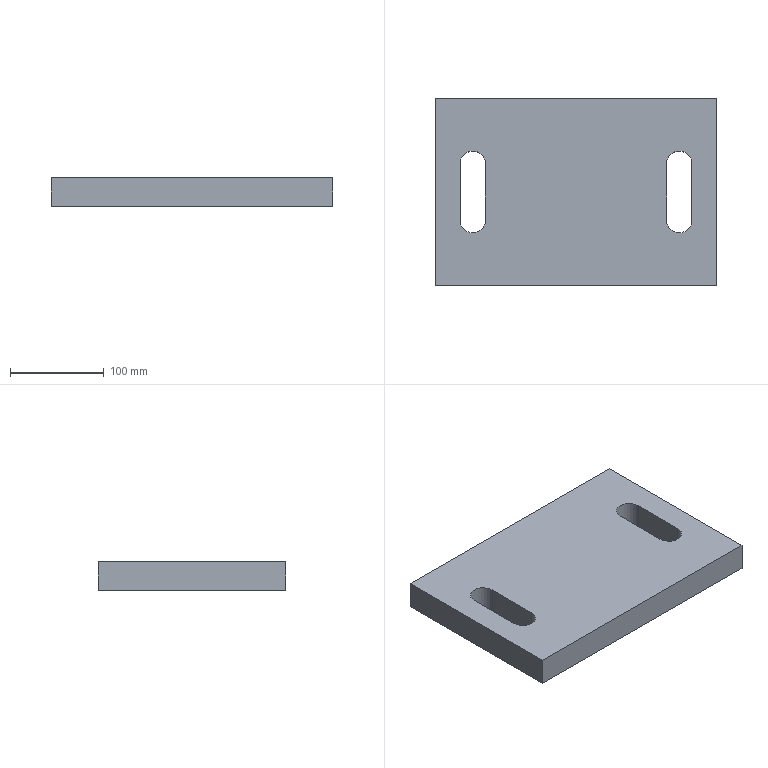Part | SolidWorks | features Extrusion 1 | 1 solid | 14 faces | box 300 x 200 x 30 mm | volume 1668447 mm3 | plane 10 | cylinder 4 | commonest cylinder face diameters 27 x4
STEP:
#1=CARTESIAN_POINT('',(273.5,130.,30.));
#2=VERTEX_POINT('',#1);
#3=CARTESIAN_POINT('',(246.5,130.,30.));
#4=VERTEX_POINT('',#3);
#5=CARTESIAN_POINT('',(260.,130.,30.));
#6=DIRECTION('',(0.,0.,1.));
#7=DIRECTION('',(1.,0.,0.));
#8=AXIS2_PLACEMENT_3D('',#5,#6,#7);
#9=CIRCLE('',#8,13.5);
#10=EDGE_CURVE('',#2,#4,#9,.T.);
#11=ORIENTED_EDGE('',*,*,#10,.F.);
#12=CARTESIAN_POINT('',(273.5,70.,30.));
#13=VERTEX_POINT('',#12);
#14=CARTESIAN_POINT('',(273.5,130.,30.));
#15=DIRECTION('',(0.,1.,0.));
#16=VECTOR('',#15,1000.);
#17=LINE('',#14,#16);
#18=EDGE_CURVE('',#13,#2,#17,.T.);
#19=ORIENTED_EDGE('',*,*,#18,.F.);
#20=CARTESIAN_POINT('',(246.5,70.,30.));
#21=VERTEX_POINT('',#20);
#22=CARTESIAN_POINT('',(260.,70.,30.));
#23=DIRECTION('',(0.,0.,1.));
#24=DIRECTION('',(1.,0.,0.));
#25=AXIS2_PLACEMENT_3D('',#22,#23,#24);
#26=CIRCLE('',#25,13.5);
#27=EDGE_CURVE('',#21,#13,#26,.T.);
#28=ORIENTED_EDGE('',*,*,#27,.F.);
#29=CARTESIAN_POINT('',(246.5,130.,30.));
#30=DIRECTION('',(0.,-1.,0.));
#31=VECTOR('',#30,1000.);
#32=LINE('',#29,#31);
#33=EDGE_CURVE('',#4,#21,#32,.T.);
#34=ORIENTED_EDGE('',*,*,#33,.F.);
#35=EDGE_LOOP('',(#11,#19,#28,#34));
#36=FACE_BOUND('',#35,.T.);
#37=CARTESIAN_POINT('',(0.,200.,30.));
#38=VERTEX_POINT('',#37);
#39=CARTESIAN_POINT('',(0.,0.,30.));
#40=VERTEX_POINT('',#39);
#41=CARTESIAN_POINT('',(0.,0.,30.));
#42=DIRECTION('',(0.,-1.,0.));
#43=VECTOR('',#42,1000.);
#44=LINE('',#41,#43);
#45=EDGE_CURVE('',#38,#40,#44,.T.);
#46=ORIENTED_EDGE('',*,*,#45,.T.);
#47=CARTESIAN_POINT('',(300.,0.,30.));
#48=VERTEX_POINT('',#47);
#49=CARTESIAN_POINT('',(0.,0.,30.));
#50=DIRECTION('',(1.,0.,0.));
#51=VECTOR('',#50,1000.);
#52=LINE('',#49,#51);
#53=EDGE_CURVE('',#40,#48,#52,.T.);
#54=ORIENTED_EDGE('',*,*,#53,.T.);
#55=CARTESIAN_POINT('',(300.,200.,30.));
#56=VERTEX_POINT('',#55);
#57=CARTESIAN_POINT('',(300.,0.,30.));
#58=DIRECTION('',(0.,1.,0.));
#59=VECTOR('',#58,1000.);
#60=LINE('',#57,#59);
#61=EDGE_CURVE('',#48,#56,#60,.T.);
#62=ORIENTED_EDGE('',*,*,#61,.T.);
#63=CARTESIAN_POINT('',(0.,200.,30.));
#64=DIRECTION('',(-1.,0.,0.));
#65=VECTOR('',#64,1000.);
#66=LINE('',#63,#65);
#67=EDGE_CURVE('',#56,#38,#66,.T.);
#68=ORIENTED_EDGE('',*,*,#67,.T.);
#69=EDGE_LOOP('',(#46,#54,#62,#68));
#70=FACE_OUTER_BOUND('',#69,.T.);
#71=CARTESIAN_POINT('',(53.5,130.,30.));
#72=VERTEX_POINT('',#71);
#73=CARTESIAN_POINT('',(26.5,130.,30.));
#74=VERTEX_POINT('',#73);
#75=CARTESIAN_POINT('',(40.,130.,30.));
#76=DIRECTION('',(0.,0.,1.));
#77=DIRECTION('',(1.,0.,0.));
#78=AXIS2_PLACEMENT_3D('',#75,#76,#77);
#79=CIRCLE('',#78,13.5);
#80=EDGE_CURVE('',#72,#74,#79,.T.);
#81=ORIENTED_EDGE('',*,*,#80,.F.);
#82=CARTESIAN_POINT('',(53.5,70.,30.));
#83=VERTEX_POINT('',#82);
#84=CARTESIAN_POINT('',(53.5,130.,30.));
#85=DIRECTION('',(0.,1.,0.));
#86=VECTOR('',#85,1000.);
#87=LINE('',#84,#86);
#88=EDGE_CURVE('',#83,#72,#87,.T.);
#89=ORIENTED_EDGE('',*,*,#88,.F.);
#90=CARTESIAN_POINT('',(26.5,70.,30.));
#91=VERTEX_POINT('',#90);
#92=CARTESIAN_POINT('',(40.,70.,30.));
#93=DIRECTION('',(0.,0.,1.));
#94=DIRECTION('',(1.,0.,0.));
#95=AXIS2_PLACEMENT_3D('',#92,#93,#94);
#96=CIRCLE('',#95,13.5);
#97=EDGE_CURVE('',#91,#83,#96,.T.);
#98=ORIENTED_EDGE('',*,*,#97,.F.);
#99=CARTESIAN_POINT('',(26.5,130.,30.));
#100=DIRECTION('',(0.,-1.,0.));
#101=VECTOR('',#100,1000.);
#102=LINE('',#99,#101);
#103=EDGE_CURVE('',#74,#91,#102,.T.);
#104=ORIENTED_EDGE('',*,*,#103,.F.);
#105=EDGE_LOOP('',(#81,#89,#98,#104));
#106=FACE_BOUND('',#105,.T.);
#107=CARTESIAN_POINT('',(0.,0.,30.));
#108=DIRECTION('',(0.,0.,-1.));
#109=DIRECTION('',(-1.,0.,0.));
#110=AXIS2_PLACEMENT_3D('',#107,#108,#109);
#111=PLANE('',#110);
#112=ADVANCED_FACE('',(#36,#70,#106),#111,.F.);
#113=CARTESIAN_POINT('',(0.,200.,0.));
#114=VERTEX_POINT('',#113);
#115=CARTESIAN_POINT('',(0.,0.,0.));
#116=VERTEX_POINT('',#115);
#117=CARTESIAN_POINT('',(0.,0.,0.));
#118=DIRECTION('',(0.,-1.,0.));
#119=VECTOR('',#118,1000.);
#120=LINE('',#117,#119);
#121=EDGE_CURVE('',#114,#116,#120,.T.);
#122=ORIENTED_EDGE('',*,*,#121,.F.);
#123=CARTESIAN_POINT('',(300.,200.,0.));
#124=VERTEX_POINT('',#123);
#125=CARTESIAN_POINT('',(0.,200.,0.));
#126=DIRECTION('',(-1.,0.,0.));
#127=VECTOR('',#126,1000.);
#128=LINE('',#125,#127);
#129=EDGE_CURVE('',#124,#114,#128,.T.);
#130=ORIENTED_EDGE('',*,*,#129,.F.);
#131=CARTESIAN_POINT('',(300.,0.,0.));
#132=VERTEX_POINT('',#131);
#133=CARTESIAN_POINT('',(300.,0.,0.));
#134=DIRECTION('',(0.,1.,0.));
#135=VECTOR('',#134,1000.);
#136=LINE('',#133,#135);
#137=EDGE_CURVE('',#132,#124,#136,.T.);
#138=ORIENTED_EDGE('',*,*,#137,.F.);
#139=CARTESIAN_POINT('',(0.,0.,0.));
#140=DIRECTION('',(1.,0.,0.));
#141=VECTOR('',#140,1000.);
#142=LINE('',#139,#141);
#143=EDGE_CURVE('',#116,#132,#142,.T.);
#144=ORIENTED_EDGE('',*,*,#143,.F.);
#145=EDGE_LOOP('',(#122,#130,#138,#144));
#146=FACE_OUTER_BOUND('',#145,.T.);
#147=CARTESIAN_POINT('',(273.5,70.,0.));
#148=VERTEX_POINT('',#147);
#149=CARTESIAN_POINT('',(273.5,130.,0.));
#150=VERTEX_POINT('',#149);
#151=CARTESIAN_POINT('',(273.5,130.,0.));
#152=DIRECTION('',(0.,1.,0.));
#153=VECTOR('',#152,1000.);
#154=LINE('',#151,#153);
#155=EDGE_CURVE('',#148,#150,#154,.T.);
#156=ORIENTED_EDGE('',*,*,#155,.T.);
#157=CARTESIAN_POINT('',(246.5,130.,0.));
#158=VERTEX_POINT('',#157);
#159=CARTESIAN_POINT('',(260.,130.,0.));
#160=DIRECTION('',(0.,0.,1.));
#161=DIRECTION('',(1.,0.,0.));
#162=AXIS2_PLACEMENT_3D('',#159,#160,#161);
#163=CIRCLE('',#162,13.5);
#164=EDGE_CURVE('',#150,#158,#163,.T.);
#165=ORIENTED_EDGE('',*,*,#164,.T.);
#166=CARTESIAN_POINT('',(246.5,70.,0.));
#167=VERTEX_POINT('',#166);
#168=CARTESIAN_POINT('',(246.5,130.,0.));
#169=DIRECTION('',(0.,-1.,0.));
#170=VECTOR('',#169,1000.);
#171=LINE('',#168,#170);
#172=EDGE_CURVE('',#158,#167,#171,.T.);
#173=ORIENTED_EDGE('',*,*,#172,.T.);
#174=CARTESIAN_POINT('',(260.,70.,0.));
#175=DIRECTION('',(0.,0.,1.));
#176=DIRECTION('',(1.,0.,0.));
#177=AXIS2_PLACEMENT_3D('',#174,#175,#176);
#178=CIRCLE('',#177,13.5);
#179=EDGE_CURVE('',#167,#148,#178,.T.);
#180=ORIENTED_EDGE('',*,*,#179,.T.);
#181=EDGE_LOOP('',(#156,#165,#173,#180));
#182=FACE_BOUND('',#181,.T.);
#183=CARTESIAN_POINT('',(53.5,70.,0.));
#184=VERTEX_POINT('',#183);
#185=CARTESIAN_POINT('',(53.5,130.,0.));
#186=VERTEX_POINT('',#185);
#187=CARTESIAN_POINT('',(53.5,130.,0.));
#188=DIRECTION('',(0.,1.,0.));
#189=VECTOR('',#188,1000.);
#190=LINE('',#187,#189);
#191=EDGE_CURVE('',#184,#186,#190,.T.);
#192=ORIENTED_EDGE('',*,*,#191,.T.);
#193=CARTESIAN_POINT('',(26.5,130.,0.));
#194=VERTEX_POINT('',#193);
#195=CARTESIAN_POINT('',(40.,130.,0.));
#196=DIRECTION('',(0.,0.,1.));
#197=DIRECTION('',(1.,0.,0.));
#198=AXIS2_PLACEMENT_3D('',#195,#196,#197);
#199=CIRCLE('',#198,13.5);
#200=EDGE_CURVE('',#186,#194,#199,.T.);
#201=ORIENTED_EDGE('',*,*,#200,.T.);
#202=CARTESIAN_POINT('',(26.5,70.,0.));
#203=VERTEX_POINT('',#202);
#204=CARTESIAN_POINT('',(26.5,130.,0.));
#205=DIRECTION('',(0.,-1.,0.));
#206=VECTOR('',#205,1000.);
#207=LINE('',#204,#206);
#208=EDGE_CURVE('',#194,#203,#207,.T.);
#209=ORIENTED_EDGE('',*,*,#208,.T.);
#210=CARTESIAN_POINT('',(40.,70.,0.));
#211=DIRECTION('',(0.,0.,1.));
#212=DIRECTION('',(1.,0.,0.));
#213=AXIS2_PLACEMENT_3D('',#210,#211,#212);
#214=CIRCLE('',#213,13.5);
#215=EDGE_CURVE('',#203,#184,#214,.T.);
#216=ORIENTED_EDGE('',*,*,#215,.T.);
#217=EDGE_LOOP('',(#192,#201,#209,#216));
#218=FACE_BOUND('',#217,.T.);
#219=CARTESIAN_POINT('',(0.,0.,0.));
#220=DIRECTION('',(0.,0.,-1.));
#221=DIRECTION('',(-1.,0.,0.));
#222=AXIS2_PLACEMENT_3D('',#219,#220,#221);
#223=PLANE('',#222);
#224=ADVANCED_FACE('',(#146,#182,#218),#223,.T.);
#225=ORIENTED_EDGE('',*,*,#121,.T.);
#226=CARTESIAN_POINT('',(0.,0.,30.));
#227=DIRECTION('',(0.,0.,-1.));
#228=VECTOR('',#227,1000.);
#229=LINE('',#226,#228);
#230=EDGE_CURVE('',#40,#116,#229,.T.);
#231=ORIENTED_EDGE('',*,*,#230,.F.);
#232=ORIENTED_EDGE('',*,*,#45,.F.);
#233=CARTESIAN_POINT('',(0.,200.,30.));
#234=DIRECTION('',(0.,0.,-1.));
#235=VECTOR('',#234,1000.);
#236=LINE('',#233,#235);
#237=EDGE_CURVE('',#38,#114,#236,.T.);
#238=ORIENTED_EDGE('',*,*,#237,.T.);
#239=EDGE_LOOP('',(#225,#231,#232,#238));
#240=FACE_OUTER_BOUND('',#239,.T.);
#241=CARTESIAN_POINT('',(0.,0.,30.));
#242=DIRECTION('',(1.,0.,0.));
#243=DIRECTION('',(0.,0.,-1.));
#244=AXIS2_PLACEMENT_3D('',#241,#242,#243);
#245=PLANE('',#244);
#246=ADVANCED_FACE('',(#240),#245,.F.);
#247=ORIENTED_EDGE('',*,*,#143,.T.);
#248=CARTESIAN_POINT('',(300.,0.,30.));
#249=DIRECTION('',(0.,0.,-1.));
#250=VECTOR('',#249,1000.);
#251=LINE('',#248,#250);
#252=EDGE_CURVE('',#48,#132,#251,.T.);
#253=ORIENTED_EDGE('',*,*,#252,.F.);
#254=ORIENTED_EDGE('',*,*,#53,.F.);
#255=ORIENTED_EDGE('',*,*,#230,.T.);
#256=EDGE_LOOP('',(#247,#253,#254,#255));
#257=FACE_OUTER_BOUND('',#256,.T.);
#258=CARTESIAN_POINT('',(0.,0.,30.));
#259=DIRECTION('',(0.,1.,0.));
#260=DIRECTION('',(0.,0.,1.));
#261=AXIS2_PLACEMENT_3D('',#258,#259,#260);
#262=PLANE('',#261);
#263=ADVANCED_FACE('',(#257),#262,.F.);
#264=ORIENTED_EDGE('',*,*,#137,.T.);
#265=CARTESIAN_POINT('',(300.,200.,30.));
#266=DIRECTION('',(0.,0.,-1.));
#267=VECTOR('',#266,1000.);
#268=LINE('',#265,#267);
#269=EDGE_CURVE('',#56,#124,#268,.T.);
#270=ORIENTED_EDGE('',*,*,#269,.F.);
#271=ORIENTED_EDGE('',*,*,#61,.F.);
#272=ORIENTED_EDGE('',*,*,#252,.T.);
#273=EDGE_LOOP('',(#264,#270,#271,#272));
#274=FACE_OUTER_BOUND('',#273,.T.);
#275=CARTESIAN_POINT('',(300.,0.,30.));
#276=DIRECTION('',(-1.,0.,0.));
#277=DIRECTION('',(0.,0.,1.));
#278=AXIS2_PLACEMENT_3D('',#275,#276,#277);
#279=PLANE('',#278);
#280=ADVANCED_FACE('',(#274),#279,.F.);
#281=ORIENTED_EDGE('',*,*,#129,.T.);
#282=ORIENTED_EDGE('',*,*,#237,.F.);
#283=ORIENTED_EDGE('',*,*,#67,.F.);
#284=ORIENTED_EDGE('',*,*,#269,.T.);
#285=EDGE_LOOP('',(#281,#282,#283,#284));
#286=FACE_OUTER_BOUND('',#285,.T.);
#287=CARTESIAN_POINT('',(0.,200.,30.));
#288=DIRECTION('',(0.,-1.,0.));
#289=DIRECTION('',(0.,0.,-1.));
#290=AXIS2_PLACEMENT_3D('',#287,#288,#289);
#291=PLANE('',#290);
#292=ADVANCED_FACE('',(#286),#291,.F.);
#293=ORIENTED_EDGE('',*,*,#164,.F.);
#294=CARTESIAN_POINT('',(273.5,130.,30.));
#295=DIRECTION('',(0.,0.,-1.));
#296=VECTOR('',#295,1000.);
#297=LINE('',#294,#296);
#298=EDGE_CURVE('',#2,#150,#297,.T.);
#299=ORIENTED_EDGE('',*,*,#298,.F.);
#300=ORIENTED_EDGE('',*,*,#10,.T.);
#301=CARTESIAN_POINT('',(246.5,130.,30.));
#302=DIRECTION('',(0.,0.,-1.));
#303=VECTOR('',#302,1000.);
#304=LINE('',#301,#303);
#305=EDGE_CURVE('',#4,#158,#304,.T.);
#306=ORIENTED_EDGE('',*,*,#305,.T.);
#307=EDGE_LOOP('',(#293,#299,#300,#306));
#308=FACE_OUTER_BOUND('',#307,.T.);
#309=CARTESIAN_POINT('',(260.,130.,30.));
#310=DIRECTION('',(0.,0.,-1.));
#311=DIRECTION('',(-1.,0.,0.));
#312=AXIS2_PLACEMENT_3D('',#309,#310,#311);
#313=CYLINDRICAL_SURFACE('',#312,13.5);
#314=ADVANCED_FACE('',(#308),#313,.F.);
#315=ORIENTED_EDGE('',*,*,#172,.F.);
#316=ORIENTED_EDGE('',*,*,#305,.F.);
#317=ORIENTED_EDGE('',*,*,#33,.T.);
#318=CARTESIAN_POINT('',(246.5,70.,30.));
#319=DIRECTION('',(0.,0.,-1.));
#320=VECTOR('',#319,1000.);
#321=LINE('',#318,#320);
#322=EDGE_CURVE('',#21,#167,#321,.T.);
#323=ORIENTED_EDGE('',*,*,#322,.T.);
#324=EDGE_LOOP('',(#315,#316,#317,#323));
#325=FACE_OUTER_BOUND('',#324,.T.);
#326=CARTESIAN_POINT('',(246.5,130.,30.));
#327=DIRECTION('',(1.,0.,0.));
#328=DIRECTION('',(0.,1.,0.));
#329=AXIS2_PLACEMENT_3D('',#326,#327,#328);
#330=PLANE('',#329);
#331=ADVANCED_FACE('',(#325),#330,.T.);
#332=ORIENTED_EDGE('',*,*,#179,.F.);
#333=ORIENTED_EDGE('',*,*,#322,.F.);
#334=ORIENTED_EDGE('',*,*,#27,.T.);
#335=CARTESIAN_POINT('',(273.5,70.,30.));
#336=DIRECTION('',(0.,0.,-1.));
#337=VECTOR('',#336,1000.);
#338=LINE('',#335,#337);
#339=EDGE_CURVE('',#13,#148,#338,.T.);
#340=ORIENTED_EDGE('',*,*,#339,.T.);
#341=EDGE_LOOP('',(#332,#333,#334,#340));
#342=FACE_OUTER_BOUND('',#341,.T.);
#343=CARTESIAN_POINT('',(260.,70.,30.));
#344=DIRECTION('',(0.,0.,-1.));
#345=DIRECTION('',(-1.,0.,0.));
#346=AXIS2_PLACEMENT_3D('',#343,#344,#345);
#347=CYLINDRICAL_SURFACE('',#346,13.5);
#348=ADVANCED_FACE('',(#342),#347,.F.);
#349=ORIENTED_EDGE('',*,*,#155,.F.);
#350=ORIENTED_EDGE('',*,*,#339,.F.);
#351=ORIENTED_EDGE('',*,*,#18,.T.);
#352=ORIENTED_EDGE('',*,*,#298,.T.);
#353=EDGE_LOOP('',(#349,#350,#351,#352));
#354=FACE_OUTER_BOUND('',#353,.T.);
#355=CARTESIAN_POINT('',(273.5,130.,30.));
#356=DIRECTION('',(-1.,0.,0.));
#357=DIRECTION('',(0.,0.,1.));
#358=AXIS2_PLACEMENT_3D('',#355,#356,#357);
#359=PLANE('',#358);
#360=ADVANCED_FACE('',(#354),#359,.T.);
#361=ORIENTED_EDGE('',*,*,#200,.F.);
#362=CARTESIAN_POINT('',(53.5,130.,30.));
#363=DIRECTION('',(0.,0.,-1.));
#364=VECTOR('',#363,1000.);
#365=LINE('',#362,#364);
#366=EDGE_CURVE('',#72,#186,#365,.T.);
#367=ORIENTED_EDGE('',*,*,#366,.F.);
#368=ORIENTED_EDGE('',*,*,#80,.T.);
#369=CARTESIAN_POINT('',(26.5,130.,30.));
#370=DIRECTION('',(0.,0.,-1.));
#371=VECTOR('',#370,1000.);
#372=LINE('',#369,#371);
#373=EDGE_CURVE('',#74,#194,#372,.T.);
#374=ORIENTED_EDGE('',*,*,#373,.T.);
#375=EDGE_LOOP('',(#361,#367,#368,#374));
#376=FACE_OUTER_BOUND('',#375,.T.);
#377=CARTESIAN_POINT('',(40.,130.,30.));
#378=DIRECTION('',(0.,0.,-1.));
#379=DIRECTION('',(-1.,0.,0.));
#380=AXIS2_PLACEMENT_3D('',#377,#378,#379);
#381=CYLINDRICAL_SURFACE('',#380,13.5);
#382=ADVANCED_FACE('',(#376),#381,.F.);
#383=ORIENTED_EDGE('',*,*,#208,.F.);
#384=ORIENTED_EDGE('',*,*,#373,.F.);
#385=ORIENTED_EDGE('',*,*,#103,.T.);
#386=CARTESIAN_POINT('',(26.5,70.,30.));
#387=DIRECTION('',(0.,0.,-1.));
#388=VECTOR('',#387,1000.);
#389=LINE('',#386,#388);
#390=EDGE_CURVE('',#91,#203,#389,.T.);
#391=ORIENTED_EDGE('',*,*,#390,.T.);
#392=EDGE_LOOP('',(#383,#384,#385,#391));
#393=FACE_OUTER_BOUND('',#392,.T.);
#394=CARTESIAN_POINT('',(26.5,130.,30.));
#395=DIRECTION('',(1.,0.,0.));
#396=DIRECTION('',(0.,1.,0.));
#397=AXIS2_PLACEMENT_3D('',#394,#395,#396);
#398=PLANE('',#397);
#399=ADVANCED_FACE('',(#393),#398,.T.);
#400=ORIENTED_EDGE('',*,*,#215,.F.);
#401=ORIENTED_EDGE('',*,*,#390,.F.);
#402=ORIENTED_EDGE('',*,*,#97,.T.);
#403=CARTESIAN_POINT('',(53.5,70.,30.));
#404=DIRECTION('',(0.,0.,-1.));
#405=VECTOR('',#404,1000.);
#406=LINE('',#403,#405);
#407=EDGE_CURVE('',#83,#184,#406,.T.);
#408=ORIENTED_EDGE('',*,*,#407,.T.);
#409=EDGE_LOOP('',(#400,#401,#402,#408));
#410=FACE_OUTER_BOUND('',#409,.T.);
#411=CARTESIAN_POINT('',(40.,70.,30.));
#412=DIRECTION('',(0.,0.,-1.));
#413=DIRECTION('',(-1.,0.,0.));
#414=AXIS2_PLACEMENT_3D('',#411,#412,#413);
#415=CYLINDRICAL_SURFACE('',#414,13.5);
#416=ADVANCED_FACE('',(#410),#415,.F.);
#417=ORIENTED_EDGE('',*,*,#191,.F.);
#418=ORIENTED_EDGE('',*,*,#407,.F.);
#419=ORIENTED_EDGE('',*,*,#88,.T.);
#420=ORIENTED_EDGE('',*,*,#366,.T.);
#421=EDGE_LOOP('',(#417,#418,#419,#420));
#422=FACE_OUTER_BOUND('',#421,.T.);
#423=CARTESIAN_POINT('',(53.5,130.,30.));
#424=DIRECTION('',(-1.,0.,0.));
#425=DIRECTION('',(0.,-1.,0.));
#426=AXIS2_PLACEMENT_3D('',#423,#424,#425);
#427=PLANE('',#426);
#428=ADVANCED_FACE('',(#422),#427,.T.);
#429=CLOSED_SHELL('',(#112,#224,#246,#263,#280,#292,#314,#331,#348,#360,#382,#399,#416,#428));
#430=MANIFOLD_SOLID_BREP('',#429);
#431=CARTESIAN_POINT('',(0.,0.,0.));
#432=DIRECTION('',(0.,0.,1.));
#433=DIRECTION('',(1.,0.,0.));
#434=AXIS2_PLACEMENT_3D('',#431,#432,#433);
#435=(LENGTH_UNIT()NAMED_UNIT(*)SI_UNIT(.MILLI.,.METRE.));
#436=UNCERTAINTY_MEASURE_WITH_UNIT(LENGTH_MEASURE(0.00001),#435,'','');
#437=(NAMED_UNIT(*)PLANE_ANGLE_UNIT()SI_UNIT($,.RADIAN.));
#438=(NAMED_UNIT(*)SI_UNIT($,.STERADIAN.)SOLID_ANGLE_UNIT());
#439=(GEOMETRIC_REPRESENTATION_CONTEXT(3)GLOBAL_UNCERTAINTY_ASSIGNED_CONTEXT((#436))GLOBAL_UNIT_ASSIGNED_CONTEXT((#435,#437,#438))REPRESENTATION_CONTEXT('',''));
#440=ADVANCED_BREP_SHAPE_REPRESENTATION('',(#430,#434),#439);